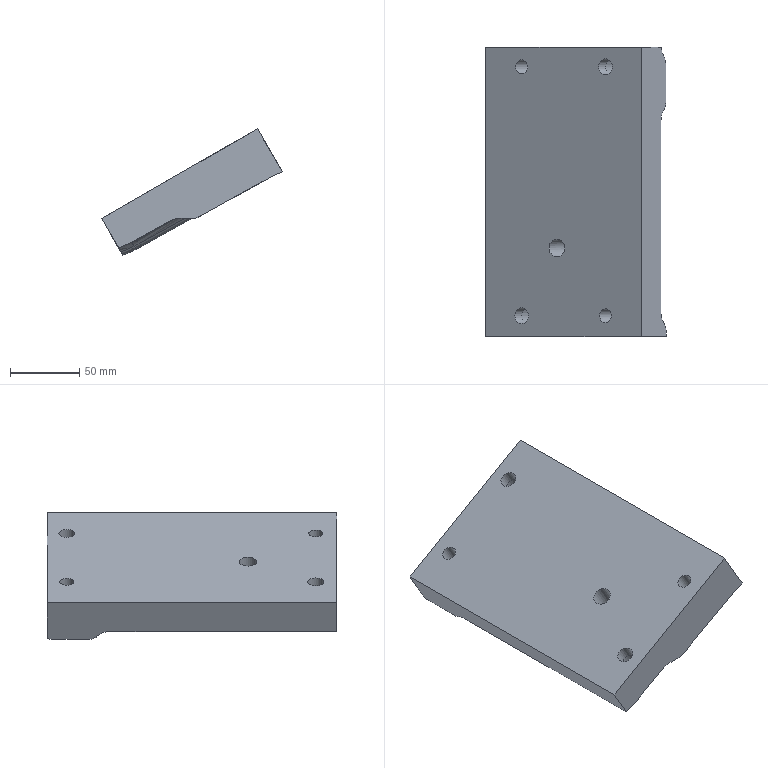Part | NX | features solid 2 | 1 solid | 63 faces | box 130.501 x 209 x 91.447 mm | volume 738276 mm3 | spline 50 | cylinder 7 | plane 6 | commonest cylinder face diameters 10 x2 11.5 x2 17.5 x2 13 x1